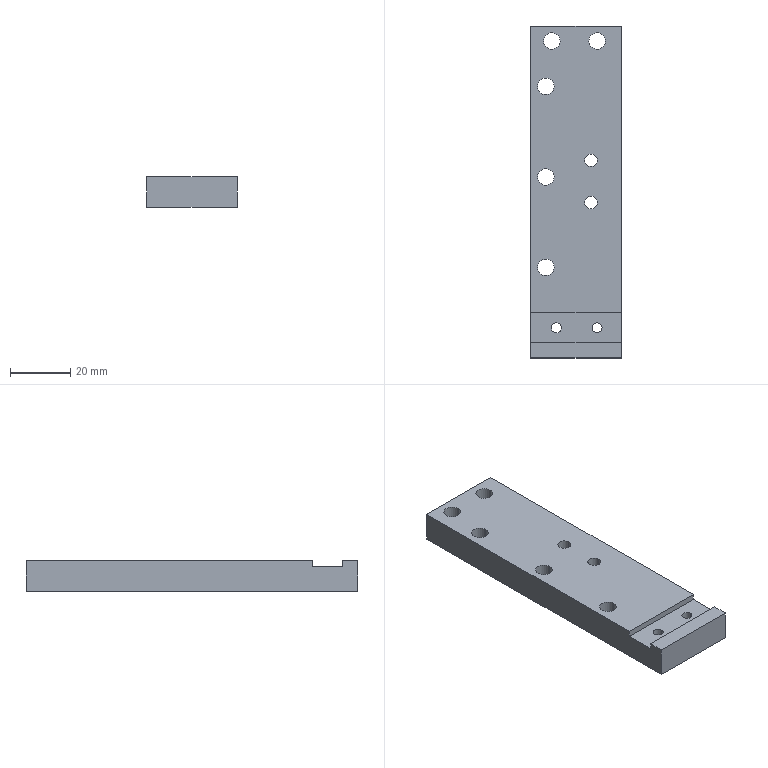Part | NX | features BREP 1 | 1 solid | 28 faces | box 30 x 110 x 10 mm | volume 30798 mm3 | cylinder 18 | plane 10 | commonest cylinder face diameters 5.5 x10 3.3 x4 4.2 x4
STEP:
#1=CARTESIAN_POINT('',(2.903,12.996,0.));
#2=VERTEX_POINT('',#1);
#3=CARTESIAN_POINT('',(7.103,12.996,0.));
#4=VERTEX_POINT('',#3);
#5=CARTESIAN_POINT('',(5.003,12.996,0.));
#6=DIRECTION('',(0.,0.,1.));
#7=DIRECTION('',(1.,0.,0.));
#8=AXIS2_PLACEMENT_3D('',#5,#6,#7);
#9=CIRCLE('',#8,2.1);
#10=EDGE_CURVE('',#2,#4,#9,.T.);
#11=ORIENTED_EDGE('',*,*,#10,.F.);
#12=CARTESIAN_POINT('',(2.903,12.996,10.));
#13=VERTEX_POINT('',#12);
#14=CARTESIAN_POINT('',(2.903,12.996,10.));
#15=DIRECTION('',(0.,0.,1.));
#16=VECTOR('',#15,1000.);
#17=LINE('',#14,#16);
#18=EDGE_CURVE('',#13,#2,#17,.F.);
#19=ORIENTED_EDGE('',*,*,#18,.F.);
#20=CARTESIAN_POINT('',(7.103,12.996,10.));
#21=VERTEX_POINT('',#20);
#22=CARTESIAN_POINT('',(5.003,12.996,10.));
#23=DIRECTION('',(0.,0.,1.));
#24=DIRECTION('',(1.,0.,0.));
#25=AXIS2_PLACEMENT_3D('',#22,#23,#24);
#26=CIRCLE('',#25,2.1);
#27=EDGE_CURVE('',#13,#21,#26,.T.);
#28=ORIENTED_EDGE('',*,*,#27,.T.);
#29=CARTESIAN_POINT('',(7.103,12.996,10.));
#30=DIRECTION('',(0.,0.,1.));
#31=VECTOR('',#30,1000.);
#32=LINE('',#29,#31);
#33=EDGE_CURVE('',#21,#4,#32,.F.);
#34=ORIENTED_EDGE('',*,*,#33,.T.);
#35=EDGE_LOOP('',(#11,#19,#28,#34));
#36=FACE_BOUND('',#35,.T.);
#37=CARTESIAN_POINT('',(5.003,12.996,10.));
#38=DIRECTION('',(0.,0.,1.));
#39=DIRECTION('',(1.,0.,0.));
#40=AXIS2_PLACEMENT_3D('',#37,#38,#39);
#41=CYLINDRICAL_SURFACE('',#40,2.1);
#42=ADVANCED_FACE('',(#36),#41,.F.);
#43=CARTESIAN_POINT('',(2.904,-1.004,0.));
#44=VERTEX_POINT('',#43);
#45=CARTESIAN_POINT('',(7.104,-1.004,0.));
#46=VERTEX_POINT('',#45);
#47=CARTESIAN_POINT('',(5.004,-1.004,0.));
#48=DIRECTION('',(0.,0.,1.));
#49=DIRECTION('',(1.,0.,0.));
#50=AXIS2_PLACEMENT_3D('',#47,#48,#49);
#51=CIRCLE('',#50,2.1);
#52=EDGE_CURVE('',#44,#46,#51,.T.);
#53=ORIENTED_EDGE('',*,*,#52,.F.);
#54=CARTESIAN_POINT('',(2.904,-1.004,10.));
#55=VERTEX_POINT('',#54);
#56=CARTESIAN_POINT('',(2.904,-1.004,10.));
#57=DIRECTION('',(0.,0.,1.));
#58=VECTOR('',#57,1000.);
#59=LINE('',#56,#58);
#60=EDGE_CURVE('',#55,#44,#59,.F.);
#61=ORIENTED_EDGE('',*,*,#60,.F.);
#62=CARTESIAN_POINT('',(7.104,-1.004,10.));
#63=VERTEX_POINT('',#62);
#64=CARTESIAN_POINT('',(5.004,-1.004,10.));
#65=DIRECTION('',(0.,0.,1.));
#66=DIRECTION('',(1.,0.,0.));
#67=AXIS2_PLACEMENT_3D('',#64,#65,#66);
#68=CIRCLE('',#67,2.1);
#69=EDGE_CURVE('',#55,#63,#68,.T.);
#70=ORIENTED_EDGE('',*,*,#69,.T.);
#71=CARTESIAN_POINT('',(7.104,-1.004,10.));
#72=DIRECTION('',(0.,0.,1.));
#73=VECTOR('',#72,1000.);
#74=LINE('',#71,#73);
#75=EDGE_CURVE('',#63,#46,#74,.F.);
#76=ORIENTED_EDGE('',*,*,#75,.T.);
#77=EDGE_LOOP('',(#53,#61,#70,#76));
#78=FACE_BOUND('',#77,.T.);
#79=CARTESIAN_POINT('',(5.004,-1.004,10.));
#80=DIRECTION('',(0.,0.,1.));
#81=DIRECTION('',(1.,0.,0.));
#82=AXIS2_PLACEMENT_3D('',#79,#80,#81);
#83=CYLINDRICAL_SURFACE('',#82,2.1);
#84=ADVANCED_FACE('',(#78),#83,.F.);
#85=CARTESIAN_POINT('',(-12.75,-22.5,0.));
#86=VERTEX_POINT('',#85);
#87=CARTESIAN_POINT('',(-7.25,-22.5,0.));
#88=VERTEX_POINT('',#87);
#89=CARTESIAN_POINT('',(-10.,-22.5,0.));
#90=DIRECTION('',(0.,0.,1.));
#91=DIRECTION('',(1.,0.,0.));
#92=AXIS2_PLACEMENT_3D('',#89,#90,#91);
#93=CIRCLE('',#92,2.75);
#94=EDGE_CURVE('',#86,#88,#93,.T.);
#95=ORIENTED_EDGE('',*,*,#94,.F.);
#96=CARTESIAN_POINT('',(-12.75,-22.5,10.));
#97=VERTEX_POINT('',#96);
#98=CARTESIAN_POINT('',(-12.75,-22.5,0.));
#99=DIRECTION('',(0.,0.,1.));
#100=VECTOR('',#99,1000.);
#101=LINE('',#98,#100);
#102=EDGE_CURVE('',#97,#86,#101,.F.);
#103=ORIENTED_EDGE('',*,*,#102,.F.);
#104=CARTESIAN_POINT('',(-7.25,-22.5,10.));
#105=VERTEX_POINT('',#104);
#106=CARTESIAN_POINT('',(-10.,-22.5,10.));
#107=DIRECTION('',(0.,0.,1.));
#108=DIRECTION('',(1.,0.,0.));
#109=AXIS2_PLACEMENT_3D('',#106,#107,#108);
#110=CIRCLE('',#109,2.75);
#111=EDGE_CURVE('',#97,#105,#110,.T.);
#112=ORIENTED_EDGE('',*,*,#111,.T.);
#113=CARTESIAN_POINT('',(-7.25,-22.5,0.));
#114=DIRECTION('',(0.,0.,1.));
#115=VECTOR('',#114,1000.);
#116=LINE('',#113,#115);
#117=EDGE_CURVE('',#105,#88,#116,.F.);
#118=ORIENTED_EDGE('',*,*,#117,.T.);
#119=EDGE_LOOP('',(#95,#103,#112,#118));
#120=FACE_BOUND('',#119,.T.);
#121=CARTESIAN_POINT('',(-10.,-22.5,0.));
#122=DIRECTION('',(0.,0.,1.));
#123=DIRECTION('',(1.,0.,0.));
#124=AXIS2_PLACEMENT_3D('',#121,#122,#123);
#125=CYLINDRICAL_SURFACE('',#124,2.75);
#126=ADVANCED_FACE('',(#120),#125,.F.);
#127=CARTESIAN_POINT('',(-12.75,7.5,0.));
#128=VERTEX_POINT('',#127);
#129=CARTESIAN_POINT('',(-7.25,7.5,0.));
#130=VERTEX_POINT('',#129);
#131=CARTESIAN_POINT('',(-10.,7.5,0.));
#132=DIRECTION('',(0.,0.,1.));
#133=DIRECTION('',(1.,0.,0.));
#134=AXIS2_PLACEMENT_3D('',#131,#132,#133);
#135=CIRCLE('',#134,2.75);
#136=EDGE_CURVE('',#128,#130,#135,.T.);
#137=ORIENTED_EDGE('',*,*,#136,.F.);
#138=CARTESIAN_POINT('',(-12.75,7.5,10.));
#139=VERTEX_POINT('',#138);
#140=CARTESIAN_POINT('',(-12.75,7.5,0.));
#141=DIRECTION('',(0.,0.,1.));
#142=VECTOR('',#141,1000.);
#143=LINE('',#140,#142);
#144=EDGE_CURVE('',#139,#128,#143,.F.);
#145=ORIENTED_EDGE('',*,*,#144,.F.);
#146=CARTESIAN_POINT('',(-7.25,7.5,10.));
#147=VERTEX_POINT('',#146);
#148=CARTESIAN_POINT('',(-10.,7.5,10.));
#149=DIRECTION('',(0.,0.,1.));
#150=DIRECTION('',(1.,0.,0.));
#151=AXIS2_PLACEMENT_3D('',#148,#149,#150);
#152=CIRCLE('',#151,2.75);
#153=EDGE_CURVE('',#139,#147,#152,.T.);
#154=ORIENTED_EDGE('',*,*,#153,.T.);
#155=CARTESIAN_POINT('',(-7.25,7.5,0.));
#156=DIRECTION('',(0.,0.,1.));
#157=VECTOR('',#156,1000.);
#158=LINE('',#155,#157);
#159=EDGE_CURVE('',#147,#130,#158,.F.);
#160=ORIENTED_EDGE('',*,*,#159,.T.);
#161=EDGE_LOOP('',(#137,#145,#154,#160));
#162=FACE_BOUND('',#161,.T.);
#163=CARTESIAN_POINT('',(-10.,7.5,0.));
#164=DIRECTION('',(0.,0.,1.));
#165=DIRECTION('',(1.,0.,0.));
#166=AXIS2_PLACEMENT_3D('',#163,#164,#165);
#167=CYLINDRICAL_SURFACE('',#166,2.75);
#168=ADVANCED_FACE('',(#162),#167,.F.);
#169=CARTESIAN_POINT('',(-12.75,37.5,0.));
#170=VERTEX_POINT('',#169);
#171=CARTESIAN_POINT('',(-7.25,37.5,0.));
#172=VERTEX_POINT('',#171);
#173=CARTESIAN_POINT('',(-10.,37.5,0.));
#174=DIRECTION('',(0.,0.,1.));
#175=DIRECTION('',(1.,0.,0.));
#176=AXIS2_PLACEMENT_3D('',#173,#174,#175);
#177=CIRCLE('',#176,2.75);
#178=EDGE_CURVE('',#170,#172,#177,.T.);
#179=ORIENTED_EDGE('',*,*,#178,.F.);
#180=CARTESIAN_POINT('',(-12.75,37.5,10.));
#181=VERTEX_POINT('',#180);
#182=CARTESIAN_POINT('',(-12.75,37.5,0.));
#183=DIRECTION('',(0.,0.,1.));
#184=VECTOR('',#183,1000.);
#185=LINE('',#182,#184);
#186=EDGE_CURVE('',#181,#170,#185,.F.);
#187=ORIENTED_EDGE('',*,*,#186,.F.);
#188=CARTESIAN_POINT('',(-7.25,37.5,10.));
#189=VERTEX_POINT('',#188);
#190=CARTESIAN_POINT('',(-10.,37.5,10.));
#191=DIRECTION('',(0.,0.,1.));
#192=DIRECTION('',(1.,0.,0.));
#193=AXIS2_PLACEMENT_3D('',#190,#191,#192);
#194=CIRCLE('',#193,2.75);
#195=EDGE_CURVE('',#181,#189,#194,.T.);
#196=ORIENTED_EDGE('',*,*,#195,.T.);
#197=CARTESIAN_POINT('',(-7.25,37.5,0.));
#198=DIRECTION('',(0.,0.,1.));
#199=VECTOR('',#198,1000.);
#200=LINE('',#197,#199);
#201=EDGE_CURVE('',#189,#172,#200,.F.);
#202=ORIENTED_EDGE('',*,*,#201,.T.);
#203=EDGE_LOOP('',(#179,#187,#196,#202));
#204=FACE_BOUND('',#203,.T.);
#205=CARTESIAN_POINT('',(-10.,37.5,0.));
#206=DIRECTION('',(0.,0.,1.));
#207=DIRECTION('',(1.,0.,0.));
#208=AXIS2_PLACEMENT_3D('',#205,#206,#207);
#209=CYLINDRICAL_SURFACE('',#208,2.75);
#210=ADVANCED_FACE('',(#204),#209,.F.);
#211=CARTESIAN_POINT('',(-8.15,-42.5,0.));
#212=VERTEX_POINT('',#211);
#213=CARTESIAN_POINT('',(-4.85,-42.5,0.));
#214=VERTEX_POINT('',#213);
#215=CARTESIAN_POINT('',(-6.5,-42.5,0.));
#216=DIRECTION('',(0.,0.,1.));
#217=DIRECTION('',(1.,0.,0.));
#218=AXIS2_PLACEMENT_3D('',#215,#216,#217);
#219=CIRCLE('',#218,1.65);
#220=EDGE_CURVE('',#212,#214,#219,.T.);
#221=ORIENTED_EDGE('',*,*,#220,.F.);
#222=CARTESIAN_POINT('',(-8.15,-42.5,8.));
#223=VERTEX_POINT('',#222);
#224=CARTESIAN_POINT('',(-8.15,-42.5,8.));
#225=DIRECTION('',(0.,0.,1.));
#226=VECTOR('',#225,1000.);
#227=LINE('',#224,#226);
#228=EDGE_CURVE('',#223,#212,#227,.F.);
#229=ORIENTED_EDGE('',*,*,#228,.F.);
#230=CARTESIAN_POINT('',(-4.85,-42.5,8.));
#231=VERTEX_POINT('',#230);
#232=CARTESIAN_POINT('',(-6.5,-42.5,8.));
#233=DIRECTION('',(0.,0.,1.));
#234=DIRECTION('',(1.,0.,0.));
#235=AXIS2_PLACEMENT_3D('',#232,#233,#234);
#236=CIRCLE('',#235,1.65);
#237=EDGE_CURVE('',#223,#231,#236,.T.);
#238=ORIENTED_EDGE('',*,*,#237,.T.);
#239=CARTESIAN_POINT('',(-4.85,-42.5,8.));
#240=DIRECTION('',(0.,0.,1.));
#241=VECTOR('',#240,1000.);
#242=LINE('',#239,#241);
#243=EDGE_CURVE('',#231,#214,#242,.F.);
#244=ORIENTED_EDGE('',*,*,#243,.T.);
#245=EDGE_LOOP('',(#221,#229,#238,#244));
#246=FACE_BOUND('',#245,.T.);
#247=CARTESIAN_POINT('',(-6.5,-42.5,8.));
#248=DIRECTION('',(0.,0.,1.));
#249=DIRECTION('',(1.,0.,0.));
#250=AXIS2_PLACEMENT_3D('',#247,#248,#249);
#251=CYLINDRICAL_SURFACE('',#250,1.65);
#252=ADVANCED_FACE('',(#246),#251,.F.);
#253=CARTESIAN_POINT('',(5.35,-42.5,0.));
#254=VERTEX_POINT('',#253);
#255=CARTESIAN_POINT('',(8.65,-42.5,0.));
#256=VERTEX_POINT('',#255);
#257=CARTESIAN_POINT('',(7.,-42.5,0.));
#258=DIRECTION('',(0.,0.,1.));
#259=DIRECTION('',(1.,0.,0.));
#260=AXIS2_PLACEMENT_3D('',#257,#258,#259);
#261=CIRCLE('',#260,1.65);
#262=EDGE_CURVE('',#254,#256,#261,.T.);
#263=ORIENTED_EDGE('',*,*,#262,.F.);
#264=CARTESIAN_POINT('',(5.35,-42.5,8.));
#265=VERTEX_POINT('',#264);
#266=CARTESIAN_POINT('',(5.35,-42.5,8.));
#267=DIRECTION('',(0.,0.,1.));
#268=VECTOR('',#267,1000.);
#269=LINE('',#266,#268);
#270=EDGE_CURVE('',#265,#254,#269,.F.);
#271=ORIENTED_EDGE('',*,*,#270,.F.);
#272=CARTESIAN_POINT('',(8.65,-42.5,8.));
#273=VERTEX_POINT('',#272);
#274=CARTESIAN_POINT('',(7.,-42.5,8.));
#275=DIRECTION('',(0.,0.,1.));
#276=DIRECTION('',(1.,0.,0.));
#277=AXIS2_PLACEMENT_3D('',#274,#275,#276);
#278=CIRCLE('',#277,1.65);
#279=EDGE_CURVE('',#265,#273,#278,.T.);
#280=ORIENTED_EDGE('',*,*,#279,.T.);
#281=CARTESIAN_POINT('',(8.65,-42.5,8.));
#282=DIRECTION('',(0.,0.,1.));
#283=VECTOR('',#282,1000.);
#284=LINE('',#281,#283);
#285=EDGE_CURVE('',#273,#256,#284,.F.);
#286=ORIENTED_EDGE('',*,*,#285,.T.);
#287=EDGE_LOOP('',(#263,#271,#280,#286));
#288=FACE_BOUND('',#287,.T.);
#289=CARTESIAN_POINT('',(7.,-42.5,8.));
#290=DIRECTION('',(0.,0.,1.));
#291=DIRECTION('',(1.,0.,0.));
#292=AXIS2_PLACEMENT_3D('',#289,#290,#291);
#293=CYLINDRICAL_SURFACE('',#292,1.65);
#294=ADVANCED_FACE('',(#288),#293,.F.);
#295=CARTESIAN_POINT('',(4.25,52.5,0.));
#296=VERTEX_POINT('',#295);
#297=CARTESIAN_POINT('',(9.75,52.5,0.));
#298=VERTEX_POINT('',#297);
#299=CARTESIAN_POINT('',(7.,52.5,0.));
#300=DIRECTION('',(0.,0.,1.));
#301=DIRECTION('',(1.,0.,0.));
#302=AXIS2_PLACEMENT_3D('',#299,#300,#301);
#303=CIRCLE('',#302,2.75);
#304=EDGE_CURVE('',#296,#298,#303,.T.);
#305=ORIENTED_EDGE('',*,*,#304,.F.);
#306=CARTESIAN_POINT('',(4.25,52.5,10.));
#307=VERTEX_POINT('',#306);
#308=CARTESIAN_POINT('',(4.25,52.5,0.));
#309=DIRECTION('',(0.,0.,1.));
#310=VECTOR('',#309,1000.);
#311=LINE('',#308,#310);
#312=EDGE_CURVE('',#307,#296,#311,.F.);
#313=ORIENTED_EDGE('',*,*,#312,.F.);
#314=CARTESIAN_POINT('',(9.75,52.5,10.));
#315=VERTEX_POINT('',#314);
#316=CARTESIAN_POINT('',(7.,52.5,10.));
#317=DIRECTION('',(0.,0.,1.));
#318=DIRECTION('',(1.,0.,0.));
#319=AXIS2_PLACEMENT_3D('',#316,#317,#318);
#320=CIRCLE('',#319,2.75);
#321=EDGE_CURVE('',#307,#315,#320,.T.);
#322=ORIENTED_EDGE('',*,*,#321,.T.);
#323=CARTESIAN_POINT('',(9.75,52.5,0.));
#324=DIRECTION('',(0.,0.,1.));
#325=VECTOR('',#324,1000.);
#326=LINE('',#323,#325);
#327=EDGE_CURVE('',#315,#298,#326,.F.);
#328=ORIENTED_EDGE('',*,*,#327,.T.);
#329=EDGE_LOOP('',(#305,#313,#322,#328));
#330=FACE_BOUND('',#329,.T.);
#331=CARTESIAN_POINT('',(7.,52.5,0.));
#332=DIRECTION('',(0.,0.,1.));
#333=DIRECTION('',(1.,0.,0.));
#334=AXIS2_PLACEMENT_3D('',#331,#332,#333);
#335=CYLINDRICAL_SURFACE('',#334,2.75);
#336=ADVANCED_FACE('',(#330),#335,.F.);
#337=CARTESIAN_POINT('',(-10.75,52.5,0.));
#338=VERTEX_POINT('',#337);
#339=CARTESIAN_POINT('',(-5.25,52.5,0.));
#340=VERTEX_POINT('',#339);
#341=CARTESIAN_POINT('',(-8.,52.5,0.));
#342=DIRECTION('',(0.,0.,1.));
#343=DIRECTION('',(1.,0.,0.));
#344=AXIS2_PLACEMENT_3D('',#341,#342,#343);
#345=CIRCLE('',#344,2.75);
#346=EDGE_CURVE('',#338,#340,#345,.T.);
#347=ORIENTED_EDGE('',*,*,#346,.F.);
#348=CARTESIAN_POINT('',(-10.75,52.5,10.));
#349=VERTEX_POINT('',#348);
#350=CARTESIAN_POINT('',(-10.75,52.5,0.));
#351=DIRECTION('',(0.,0.,1.));
#352=VECTOR('',#351,1000.);
#353=LINE('',#350,#352);
#354=EDGE_CURVE('',#349,#338,#353,.F.);
#355=ORIENTED_EDGE('',*,*,#354,.F.);
#356=CARTESIAN_POINT('',(-5.25,52.5,10.));
#357=VERTEX_POINT('',#356);
#358=CARTESIAN_POINT('',(-8.,52.5,10.));
#359=DIRECTION('',(0.,0.,1.));
#360=DIRECTION('',(1.,0.,0.));
#361=AXIS2_PLACEMENT_3D('',#358,#359,#360);
#362=CIRCLE('',#361,2.75);
#363=EDGE_CURVE('',#349,#357,#362,.T.);
#364=ORIENTED_EDGE('',*,*,#363,.T.);
#365=CARTESIAN_POINT('',(-5.25,52.5,0.));
#366=DIRECTION('',(0.,0.,1.));
#367=VECTOR('',#366,1000.);
#368=LINE('',#365,#367);
#369=EDGE_CURVE('',#357,#340,#368,.F.);
#370=ORIENTED_EDGE('',*,*,#369,.T.);
#371=EDGE_LOOP('',(#347,#355,#364,#370));
#372=FACE_BOUND('',#371,.T.);
#373=CARTESIAN_POINT('',(-8.,52.5,0.));
#374=DIRECTION('',(0.,0.,1.));
#375=DIRECTION('',(1.,0.,0.));
#376=AXIS2_PLACEMENT_3D('',#373,#374,#375);
#377=CYLINDRICAL_SURFACE('',#376,2.75);
#378=ADVANCED_FACE('',(#372),#377,.F.);
#379=CARTESIAN_POINT('',(15.,-37.5,10.));
#380=VERTEX_POINT('',#379);
#381=CARTESIAN_POINT('',(-15.,-37.5,10.));
#382=VERTEX_POINT('',#381);
#383=CARTESIAN_POINT('',(-15.,-37.5,10.));
#384=DIRECTION('',(-1.,0.,0.));
#385=VECTOR('',#384,1000.);
#386=LINE('',#383,#385);
#387=EDGE_CURVE('',#380,#382,#386,.T.);
#388=ORIENTED_EDGE('',*,*,#387,.F.);
#389=CARTESIAN_POINT('',(15.,57.5,10.));
#390=VERTEX_POINT('',#389);
#391=CARTESIAN_POINT('',(15.,57.5,10.));
#392=DIRECTION('',(0.,1.,0.));
#393=VECTOR('',#392,1000.);
#394=LINE('',#391,#393);
#395=EDGE_CURVE('',#380,#390,#394,.T.);
#396=ORIENTED_EDGE('',*,*,#395,.T.);
#397=CARTESIAN_POINT('',(-15.,57.5,10.));
#398=VERTEX_POINT('',#397);
#399=CARTESIAN_POINT('',(-15.,57.5,10.));
#400=DIRECTION('',(-1.,0.,0.));
#401=VECTOR('',#400,1000.);
#402=LINE('',#399,#401);
#403=EDGE_CURVE('',#390,#398,#402,.T.);
#404=ORIENTED_EDGE('',*,*,#403,.T.);
#405=CARTESIAN_POINT('',(-15.,57.5,10.));
#406=DIRECTION('',(0.,-1.,0.));
#407=VECTOR('',#406,1000.);
#408=LINE('',#405,#407);
#409=EDGE_CURVE('',#398,#382,#408,.T.);
#410=ORIENTED_EDGE('',*,*,#409,.T.);
#411=EDGE_LOOP('',(#388,#396,#404,#410));
#412=FACE_BOUND('',#411,.T.);
#413=CARTESIAN_POINT('',(5.003,12.996,10.));
#414=DIRECTION('',(0.,0.,1.));
#415=DIRECTION('',(1.,0.,0.));
#416=AXIS2_PLACEMENT_3D('',#413,#414,#415);
#417=CIRCLE('',#416,2.1);
#418=EDGE_CURVE('',#21,#13,#417,.T.);
#419=ORIENTED_EDGE('',*,*,#418,.F.);
#420=ORIENTED_EDGE('',*,*,#27,.F.);
#421=EDGE_LOOP('',(#419,#420));
#422=FACE_BOUND('',#421,.T.);
#423=CARTESIAN_POINT('',(5.004,-1.004,10.));
#424=DIRECTION('',(0.,0.,1.));
#425=DIRECTION('',(1.,0.,0.));
#426=AXIS2_PLACEMENT_3D('',#423,#424,#425);
#427=CIRCLE('',#426,2.1);
#428=EDGE_CURVE('',#63,#55,#427,.T.);
#429=ORIENTED_EDGE('',*,*,#428,.F.);
#430=ORIENTED_EDGE('',*,*,#69,.F.);
#431=EDGE_LOOP('',(#429,#430));
#432=FACE_BOUND('',#431,.T.);
#433=CARTESIAN_POINT('',(-10.,-22.5,10.));
#434=DIRECTION('',(0.,0.,1.));
#435=DIRECTION('',(1.,0.,0.));
#436=AXIS2_PLACEMENT_3D('',#433,#434,#435);
#437=CIRCLE('',#436,2.75);
#438=EDGE_CURVE('',#105,#97,#437,.T.);
#439=ORIENTED_EDGE('',*,*,#438,.F.);
#440=ORIENTED_EDGE('',*,*,#111,.F.);
#441=EDGE_LOOP('',(#439,#440));
#442=FACE_BOUND('',#441,.T.);
#443=CARTESIAN_POINT('',(-10.,7.5,10.));
#444=DIRECTION('',(0.,0.,1.));
#445=DIRECTION('',(1.,0.,0.));
#446=AXIS2_PLACEMENT_3D('',#443,#444,#445);
#447=CIRCLE('',#446,2.75);
#448=EDGE_CURVE('',#147,#139,#447,.T.);
#449=ORIENTED_EDGE('',*,*,#448,.F.);
#450=ORIENTED_EDGE('',*,*,#153,.F.);
#451=EDGE_LOOP('',(#449,#450));
#452=FACE_BOUND('',#451,.T.);
#453=CARTESIAN_POINT('',(-10.,37.5,10.));
#454=DIRECTION('',(0.,0.,1.));
#455=DIRECTION('',(1.,0.,0.));
#456=AXIS2_PLACEMENT_3D('',#453,#454,#455);
#457=CIRCLE('',#456,2.75);
#458=EDGE_CURVE('',#189,#181,#457,.T.);
#459=ORIENTED_EDGE('',*,*,#458,.F.);
#460=ORIENTED_EDGE('',*,*,#195,.F.);
#461=EDGE_LOOP('',(#459,#460));
#462=FACE_BOUND('',#461,.T.);
#463=CARTESIAN_POINT('',(7.,52.5,10.));
#464=DIRECTION('',(0.,0.,1.));
#465=DIRECTION('',(1.,0.,0.));
#466=AXIS2_PLACEMENT_3D('',#463,#464,#465);
#467=CIRCLE('',#466,2.75);
#468=EDGE_CURVE('',#315,#307,#467,.T.);
#469=ORIENTED_EDGE('',*,*,#468,.F.);
#470=ORIENTED_EDGE('',*,*,#321,.F.);
#471=EDGE_LOOP('',(#469,#470));
#472=FACE_BOUND('',#471,.T.);
#473=CARTESIAN_POINT('',(-8.,52.5,10.));
#474=DIRECTION('',(0.,0.,1.));
#475=DIRECTION('',(1.,0.,0.));
#476=AXIS2_PLACEMENT_3D('',#473,#474,#475);
#477=CIRCLE('',#476,2.75);
#478=EDGE_CURVE('',#357,#349,#477,.T.);
#479=ORIENTED_EDGE('',*,*,#478,.F.);
#480=ORIENTED_EDGE('',*,*,#363,.F.);
#481=EDGE_LOOP('',(#479,#480));
#482=FACE_BOUND('',#481,.T.);
#483=CARTESIAN_POINT('',(-15.,-52.5,10.));
#484=DIRECTION('',(0.,0.,1.));
#485=DIRECTION('',(1.,0.,0.));
#486=AXIS2_PLACEMENT_3D('',#483,#484,#485);
#487=PLANE('',#486);
#488=ADVANCED_FACE('',(#412,#422,#432,#442,#452,#462,#472,#482),#487,.T.);
#489=CARTESIAN_POINT('',(-15.,-37.5,8.));
#490=VERTEX_POINT('',#489);
#491=CARTESIAN_POINT('',(-15.,-47.5,8.));
#492=VERTEX_POINT('',#491);
#493=CARTESIAN_POINT('',(-15.,-37.5,8.));
#494=DIRECTION('',(0.,-1.,0.));
#495=VECTOR('',#494,1000.);
#496=LINE('',#493,#495);
#497=EDGE_CURVE('',#490,#492,#496,.T.);
#498=ORIENTED_EDGE('',*,*,#497,.F.);
#499=CARTESIAN_POINT('',(-15.,-37.5,8.));
#500=DIRECTION('',(0.,0.,1.));
#501=VECTOR('',#500,1000.);
#502=LINE('',#499,#501);
#503=EDGE_CURVE('',#490,#382,#502,.T.);
#504=ORIENTED_EDGE('',*,*,#503,.T.);
#505=ORIENTED_EDGE('',*,*,#409,.F.);
#506=CARTESIAN_POINT('',(-15.,57.5,0.));
#507=VERTEX_POINT('',#506);
#508=CARTESIAN_POINT('',(-15.,57.5,10.));
#509=DIRECTION('',(0.,0.,-1.));
#510=VECTOR('',#509,1000.);
#511=LINE('',#508,#510);
#512=EDGE_CURVE('',#398,#507,#511,.T.);
#513=ORIENTED_EDGE('',*,*,#512,.T.);
#514=CARTESIAN_POINT('',(-15.,-52.5,0.));
#515=VERTEX_POINT('',#514);
#516=CARTESIAN_POINT('',(-15.,57.5,0.));
#517=DIRECTION('',(0.,-1.,0.));
#518=VECTOR('',#517,1000.);
#519=LINE('',#516,#518);
#520=EDGE_CURVE('',#507,#515,#519,.T.);
#521=ORIENTED_EDGE('',*,*,#520,.T.);
#522=CARTESIAN_POINT('',(-15.,-52.5,10.));
#523=VERTEX_POINT('',#522);
#524=CARTESIAN_POINT('',(-15.,-52.5,10.));
#525=DIRECTION('',(0.,0.,-1.));
#526=VECTOR('',#525,1000.);
#527=LINE('',#524,#526);
#528=EDGE_CURVE('',#523,#515,#527,.T.);
#529=ORIENTED_EDGE('',*,*,#528,.F.);
#530=CARTESIAN_POINT('',(-15.,-47.5,10.));
#531=VERTEX_POINT('',#530);
#532=CARTESIAN_POINT('',(-15.,57.5,10.));
#533=DIRECTION('',(0.,-1.,0.));
#534=VECTOR('',#533,1000.);
#535=LINE('',#532,#534);
#536=EDGE_CURVE('',#531,#523,#535,.T.);
#537=ORIENTED_EDGE('',*,*,#536,.F.);
#538=CARTESIAN_POINT('',(-15.,-47.5,8.));
#539=DIRECTION('',(0.,0.,1.));
#540=VECTOR('',#539,1000.);
#541=LINE('',#538,#540);
#542=EDGE_CURVE('',#492,#531,#541,.T.);
#543=ORIENTED_EDGE('',*,*,#542,.F.);
#544=EDGE_LOOP('',(#498,#504,#505,#513,#521,#529,#537,#543));
#545=FACE_BOUND('',#544,.T.);
#546=CARTESIAN_POINT('',(-15.,57.5,10.));
#547=DIRECTION('',(1.,0.,0.));
#548=DIRECTION('',(0.,1.,0.));
#549=AXIS2_PLACEMENT_3D('',#546,#547,#548);
#550=PLANE('',#549);
#551=ADVANCED_FACE('',(#545),#550,.F.);
#552=CARTESIAN_POINT('',(15.,-52.5,0.));
#553=VERTEX_POINT('',#552);
#554=CARTESIAN_POINT('',(-15.,-52.5,0.));
#555=DIRECTION('',(1.,0.,0.));
#556=VECTOR('',#555,1000.);
#557=LINE('',#554,#556);
#558=EDGE_CURVE('',#515,#553,#557,.T.);
#559=ORIENTED_EDGE('',*,*,#558,.T.);
#560=CARTESIAN_POINT('',(15.,-52.5,10.));
#561=VERTEX_POINT('',#560);
#562=CARTESIAN_POINT('',(15.,-52.5,10.));
#563=DIRECTION('',(0.,0.,-1.));
#564=VECTOR('',#563,1000.);
#565=LINE('',#562,#564);
#566=EDGE_CURVE('',#561,#553,#565,.T.);
#567=ORIENTED_EDGE('',*,*,#566,.F.);
#568=CARTESIAN_POINT('',(-15.,-52.5,10.));
#569=DIRECTION('',(1.,0.,0.));
#570=VECTOR('',#569,1000.);
#571=LINE('',#568,#570);
#572=EDGE_CURVE('',#523,#561,#571,.T.);
#573=ORIENTED_EDGE('',*,*,#572,.F.);
#574=ORIENTED_EDGE('',*,*,#528,.T.);
#575=EDGE_LOOP('',(#559,#567,#573,#574));
#576=FACE_BOUND('',#575,.T.);
#577=CARTESIAN_POINT('',(-15.,-52.5,10.));
#578=DIRECTION('',(0.,1.,0.));
#579=DIRECTION('',(1.,0.,0.));
#580=AXIS2_PLACEMENT_3D('',#577,#578,#579);
#581=PLANE('',#580);
#582=ADVANCED_FACE('',(#576),#581,.F.);
#583=ORIENTED_EDGE('',*,*,#395,.F.);
#584=CARTESIAN_POINT('',(15.,-37.5,8.));
#585=VERTEX_POINT('',#584);
#586=CARTESIAN_POINT('',(15.,-37.5,8.));
#587=DIRECTION('',(0.,0.,1.));
#588=VECTOR('',#587,1000.);
#589=LINE('',#586,#588);
#590=EDGE_CURVE('',#585,#380,#589,.T.);
#591=ORIENTED_EDGE('',*,*,#590,.F.);
#592=CARTESIAN_POINT('',(15.,-47.5,8.));
#593=VERTEX_POINT('',#592);
#594=CARTESIAN_POINT('',(15.,-37.5,8.));
#595=DIRECTION('',(0.,1.,0.));
#596=VECTOR('',#595,1000.);
#597=LINE('',#594,#596);
#598=EDGE_CURVE('',#593,#585,#597,.T.);
#599=ORIENTED_EDGE('',*,*,#598,.F.);
#600=CARTESIAN_POINT('',(15.,-47.5,10.));
#601=VERTEX_POINT('',#600);
#602=CARTESIAN_POINT('',(15.,-47.5,8.));
#603=DIRECTION('',(0.,0.,1.));
#604=VECTOR('',#603,1000.);
#605=LINE('',#602,#604);
#606=EDGE_CURVE('',#593,#601,#605,.T.);
#607=ORIENTED_EDGE('',*,*,#606,.T.);
#608=CARTESIAN_POINT('',(15.,57.5,10.));
#609=DIRECTION('',(0.,1.,0.));
#610=VECTOR('',#609,1000.);
#611=LINE('',#608,#610);
#612=EDGE_CURVE('',#561,#601,#611,.T.);
#613=ORIENTED_EDGE('',*,*,#612,.F.);
#614=ORIENTED_EDGE('',*,*,#566,.T.);
#615=CARTESIAN_POINT('',(15.,57.5,0.));
#616=VERTEX_POINT('',#615);
#617=CARTESIAN_POINT('',(15.,57.5,0.));
#618=DIRECTION('',(0.,1.,0.));
#619=VECTOR('',#618,1000.);
#620=LINE('',#617,#619);
#621=EDGE_CURVE('',#553,#616,#620,.T.);
#622=ORIENTED_EDGE('',*,*,#621,.T.);
#623=CARTESIAN_POINT('',(15.,57.5,10.));
#624=DIRECTION('',(0.,0.,-1.));
#625=VECTOR('',#624,1000.);
#626=LINE('',#623,#625);
#627=EDGE_CURVE('',#390,#616,#626,.T.);
#628=ORIENTED_EDGE('',*,*,#627,.F.);
#629=EDGE_LOOP('',(#583,#591,#599,#607,#613,#614,#622,#628));
#630=FACE_BOUND('',#629,.T.);
#631=CARTESIAN_POINT('',(15.,57.5,10.));
#632=DIRECTION('',(-1.,0.,0.));
#633=DIRECTION('',(0.,1.,0.));
#634=AXIS2_PLACEMENT_3D('',#631,#632,#633);
#635=PLANE('',#634);
#636=ADVANCED_FACE('',(#630),#635,.F.);
#637=CARTESIAN_POINT('',(-15.,57.5,0.));
#638=DIRECTION('',(-1.,0.,0.));
#639=VECTOR('',#638,1000.);
#640=LINE('',#637,#639);
#641=EDGE_CURVE('',#616,#507,#640,.T.);
#642=ORIENTED_EDGE('',*,*,#641,.T.);
#643=ORIENTED_EDGE('',*,*,#512,.F.);
#644=ORIENTED_EDGE('',*,*,#403,.F.);
#645=ORIENTED_EDGE('',*,*,#627,.T.);
#646=EDGE_LOOP('',(#642,#643,#644,#645));
#647=FACE_BOUND('',#646,.T.);
#648=CARTESIAN_POINT('',(-15.,57.5,10.));
#649=DIRECTION('',(0.,-1.,0.));
#650=DIRECTION('',(0.,0.,-1.));
#651=AXIS2_PLACEMENT_3D('',#648,#649,#650);
#652=PLANE('',#651);
#653=ADVANCED_FACE('',(#647),#652,.F.);
#654=CARTESIAN_POINT('',(-15.,-47.5,10.));
#655=DIRECTION('',(1.,0.,0.));
#656=VECTOR('',#655,1000.);
#657=LINE('',#654,#656);
#658=EDGE_CURVE('',#531,#601,#657,.T.);
#659=ORIENTED_EDGE('',*,*,#658,.F.);
#660=ORIENTED_EDGE('',*,*,#536,.T.);
#661=ORIENTED_EDGE('',*,*,#572,.T.);
#662=ORIENTED_EDGE('',*,*,#612,.T.);
#663=EDGE_LOOP('',(#659,#660,#661,#662));
#664=FACE_BOUND('',#663,.T.);
#665=CARTESIAN_POINT('',(-15.,-52.5,10.));
#666=DIRECTION('',(0.,0.,1.));
#667=DIRECTION('',(1.,0.,0.));
#668=AXIS2_PLACEMENT_3D('',#665,#666,#667);
#669=PLANE('',#668);
#670=ADVANCED_FACE('',(#664),#669,.T.);
#671=ORIENTED_EDGE('',*,*,#520,.F.);
#672=ORIENTED_EDGE('',*,*,#641,.F.);
#673=ORIENTED_EDGE('',*,*,#621,.F.);
#674=ORIENTED_EDGE('',*,*,#558,.F.);
#675=EDGE_LOOP('',(#671,#672,#673,#674));
#676=FACE_BOUND('',#675,.T.);
#677=CARTESIAN_POINT('',(5.003,12.996,0.));
#678=DIRECTION('',(0.,0.,1.));
#679=DIRECTION('',(1.,0.,0.));
#680=AXIS2_PLACEMENT_3D('',#677,#678,#679);
#681=CIRCLE('',#680,2.1);
#682=EDGE_CURVE('',#4,#2,#681,.T.);
#683=ORIENTED_EDGE('',*,*,#682,.T.);
#684=ORIENTED_EDGE('',*,*,#10,.T.);
#685=EDGE_LOOP('',(#683,#684));
#686=FACE_BOUND('',#685,.T.);
#687=CARTESIAN_POINT('',(5.004,-1.004,0.));
#688=DIRECTION('',(0.,0.,1.));
#689=DIRECTION('',(1.,0.,0.));
#690=AXIS2_PLACEMENT_3D('',#687,#688,#689);
#691=CIRCLE('',#690,2.1);
#692=EDGE_CURVE('',#46,#44,#691,.T.);
#693=ORIENTED_EDGE('',*,*,#692,.T.);
#694=ORIENTED_EDGE('',*,*,#52,.T.);
#695=EDGE_LOOP('',(#693,#694));
#696=FACE_BOUND('',#695,.T.);
#697=CARTESIAN_POINT('',(-10.,-22.5,0.));
#698=DIRECTION('',(0.,0.,1.));
#699=DIRECTION('',(1.,0.,0.));
#700=AXIS2_PLACEMENT_3D('',#697,#698,#699);
#701=CIRCLE('',#700,2.75);
#702=EDGE_CURVE('',#88,#86,#701,.T.);
#703=ORIENTED_EDGE('',*,*,#702,.T.);
#704=ORIENTED_EDGE('',*,*,#94,.T.);
#705=EDGE_LOOP('',(#703,#704));
#706=FACE_BOUND('',#705,.T.);
#707=CARTESIAN_POINT('',(-10.,7.5,0.));
#708=DIRECTION('',(0.,0.,1.));
#709=DIRECTION('',(1.,0.,0.));
#710=AXIS2_PLACEMENT_3D('',#707,#708,#709);
#711=CIRCLE('',#710,2.75);
#712=EDGE_CURVE('',#130,#128,#711,.T.);
#713=ORIENTED_EDGE('',*,*,#712,.T.);
#714=ORIENTED_EDGE('',*,*,#136,.T.);
#715=EDGE_LOOP('',(#713,#714));
#716=FACE_BOUND('',#715,.T.);
#717=CARTESIAN_POINT('',(-10.,37.5,0.));
#718=DIRECTION('',(0.,0.,1.));
#719=DIRECTION('',(1.,0.,0.));
#720=AXIS2_PLACEMENT_3D('',#717,#718,#719);
#721=CIRCLE('',#720,2.75);
#722=EDGE_CURVE('',#172,#170,#721,.T.);
#723=ORIENTED_EDGE('',*,*,#722,.T.);
#724=ORIENTED_EDGE('',*,*,#178,.T.);
#725=EDGE_LOOP('',(#723,#724));
#726=FACE_BOUND('',#725,.T.);
#727=CARTESIAN_POINT('',(-6.5,-42.5,0.));
#728=DIRECTION('',(0.,0.,1.));
#729=DIRECTION('',(1.,0.,0.));
#730=AXIS2_PLACEMENT_3D('',#727,#728,#729);
#731=CIRCLE('',#730,1.65);
#732=EDGE_CURVE('',#214,#212,#731,.T.);
#733=ORIENTED_EDGE('',*,*,#732,.T.);
#734=ORIENTED_EDGE('',*,*,#220,.T.);
#735=EDGE_LOOP('',(#733,#734));
#736=FACE_BOUND('',#735,.T.);
#737=CARTESIAN_POINT('',(7.,-42.5,0.));
#738=DIRECTION('',(0.,0.,1.));
#739=DIRECTION('',(1.,0.,0.));
#740=AXIS2_PLACEMENT_3D('',#737,#738,#739);
#741=CIRCLE('',#740,1.65);
#742=EDGE_CURVE('',#256,#254,#741,.T.);
#743=ORIENTED_EDGE('',*,*,#742,.T.);
#744=ORIENTED_EDGE('',*,*,#262,.T.);
#745=EDGE_LOOP('',(#743,#744));
#746=FACE_BOUND('',#745,.T.);
#747=CARTESIAN_POINT('',(7.,52.5,0.));
#748=DIRECTION('',(0.,0.,1.));
#749=DIRECTION('',(1.,0.,0.));
#750=AXIS2_PLACEMENT_3D('',#747,#748,#749);
#751=CIRCLE('',#750,2.75);
#752=EDGE_CURVE('',#298,#296,#751,.T.);
#753=ORIENTED_EDGE('',*,*,#752,.T.);
#754=ORIENTED_EDGE('',*,*,#304,.T.);
#755=EDGE_LOOP('',(#753,#754));
#756=FACE_BOUND('',#755,.T.);
#757=CARTESIAN_POINT('',(-8.,52.5,0.));
#758=DIRECTION('',(0.,0.,1.));
#759=DIRECTION('',(1.,0.,0.));
#760=AXIS2_PLACEMENT_3D('',#757,#758,#759);
#761=CIRCLE('',#760,2.75);
#762=EDGE_CURVE('',#340,#338,#761,.T.);
#763=ORIENTED_EDGE('',*,*,#762,.T.);
#764=ORIENTED_EDGE('',*,*,#346,.T.);
#765=EDGE_LOOP('',(#763,#764));
#766=FACE_BOUND('',#765,.T.);
#767=CARTESIAN_POINT('',(-15.,-52.5,0.));
#768=DIRECTION('',(0.,0.,1.));
#769=DIRECTION('',(1.,0.,0.));
#770=AXIS2_PLACEMENT_3D('',#767,#768,#769);
#771=PLANE('',#770);
#772=ADVANCED_FACE('',(#676,#686,#696,#706,#716,#726,#736,#746,#756,#766),#771,.F.);
#773=ORIENTED_EDGE('',*,*,#387,.T.);
#774=ORIENTED_EDGE('',*,*,#503,.F.);
#775=CARTESIAN_POINT('',(-15.,-37.5,8.));
#776=DIRECTION('',(-1.,0.,0.));
#777=VECTOR('',#776,1000.);
#778=LINE('',#775,#777);
#779=EDGE_CURVE('',#585,#490,#778,.T.);
#780=ORIENTED_EDGE('',*,*,#779,.F.);
#781=ORIENTED_EDGE('',*,*,#590,.T.);
#782=EDGE_LOOP('',(#773,#774,#780,#781));
#783=FACE_BOUND('',#782,.T.);
#784=CARTESIAN_POINT('',(-15.,-37.5,8.));
#785=DIRECTION('',(0.,1.,0.));
#786=DIRECTION('',(1.,0.,0.));
#787=AXIS2_PLACEMENT_3D('',#784,#785,#786);
#788=PLANE('',#787);
#789=ADVANCED_FACE('',(#783),#788,.F.);
#790=ORIENTED_EDGE('',*,*,#658,.T.);
#791=ORIENTED_EDGE('',*,*,#606,.F.);
#792=CARTESIAN_POINT('',(-15.,-47.5,8.));
#793=DIRECTION('',(1.,0.,0.));
#794=VECTOR('',#793,1000.);
#795=LINE('',#792,#794);
#796=EDGE_CURVE('',#492,#593,#795,.T.);
#797=ORIENTED_EDGE('',*,*,#796,.F.);
#798=ORIENTED_EDGE('',*,*,#542,.T.);
#799=EDGE_LOOP('',(#790,#791,#797,#798));
#800=FACE_BOUND('',#799,.T.);
#801=CARTESIAN_POINT('',(-15.,-47.5,8.));
#802=DIRECTION('',(0.,-1.,0.));
#803=DIRECTION('',(0.,0.,-1.));
#804=AXIS2_PLACEMENT_3D('',#801,#802,#803);
#805=PLANE('',#804);
#806=ADVANCED_FACE('',(#800),#805,.F.);
#807=ORIENTED_EDGE('',*,*,#497,.T.);
#808=ORIENTED_EDGE('',*,*,#796,.T.);
#809=ORIENTED_EDGE('',*,*,#598,.T.);
#810=ORIENTED_EDGE('',*,*,#779,.T.);
#811=EDGE_LOOP('',(#807,#808,#809,#810));
#812=FACE_BOUND('',#811,.T.);
#813=CARTESIAN_POINT('',(-6.5,-42.5,8.));
#814=DIRECTION('',(0.,0.,1.));
#815=DIRECTION('',(1.,0.,0.));
#816=AXIS2_PLACEMENT_3D('',#813,#814,#815);
#817=CIRCLE('',#816,1.65);
#818=EDGE_CURVE('',#231,#223,#817,.T.);
#819=ORIENTED_EDGE('',*,*,#818,.F.);
#820=ORIENTED_EDGE('',*,*,#237,.F.);
#821=EDGE_LOOP('',(#819,#820));
#822=FACE_BOUND('',#821,.T.);
#823=CARTESIAN_POINT('',(7.,-42.5,8.));
#824=DIRECTION('',(0.,0.,1.));
#825=DIRECTION('',(1.,0.,0.));
#826=AXIS2_PLACEMENT_3D('',#823,#824,#825);
#827=CIRCLE('',#826,1.65);
#828=EDGE_CURVE('',#273,#265,#827,.T.);
#829=ORIENTED_EDGE('',*,*,#828,.F.);
#830=ORIENTED_EDGE('',*,*,#279,.F.);
#831=EDGE_LOOP('',(#829,#830));
#832=FACE_BOUND('',#831,.T.);
#833=CARTESIAN_POINT('',(-15.,-47.5,8.));
#834=DIRECTION('',(0.,0.,1.));
#835=DIRECTION('',(1.,0.,0.));
#836=AXIS2_PLACEMENT_3D('',#833,#834,#835);
#837=PLANE('',#836);
#838=ADVANCED_FACE('',(#812,#822,#832),#837,.T.);
#839=ORIENTED_EDGE('',*,*,#354,.T.);
#840=ORIENTED_EDGE('',*,*,#762,.F.);
#841=ORIENTED_EDGE('',*,*,#369,.F.);
#842=ORIENTED_EDGE('',*,*,#478,.T.);
#843=EDGE_LOOP('',(#839,#840,#841,#842));
#844=FACE_BOUND('',#843,.T.);
#845=CARTESIAN_POINT('',(-8.,52.5,0.));
#846=DIRECTION('',(0.,0.,1.));
#847=DIRECTION('',(1.,0.,0.));
#848=AXIS2_PLACEMENT_3D('',#845,#846,#847);
#849=CYLINDRICAL_SURFACE('',#848,2.75);
#850=ADVANCED_FACE('',(#844),#849,.F.);
#851=ORIENTED_EDGE('',*,*,#312,.T.);
#852=ORIENTED_EDGE('',*,*,#752,.F.);
#853=ORIENTED_EDGE('',*,*,#327,.F.);
#854=ORIENTED_EDGE('',*,*,#468,.T.);
#855=EDGE_LOOP('',(#851,#852,#853,#854));
#856=FACE_BOUND('',#855,.T.);
#857=CARTESIAN_POINT('',(7.,52.5,0.));
#858=DIRECTION('',(0.,0.,1.));
#859=DIRECTION('',(1.,0.,0.));
#860=AXIS2_PLACEMENT_3D('',#857,#858,#859);
#861=CYLINDRICAL_SURFACE('',#860,2.75);
#862=ADVANCED_FACE('',(#856),#861,.F.);
#863=ORIENTED_EDGE('',*,*,#270,.T.);
#864=ORIENTED_EDGE('',*,*,#742,.F.);
#865=ORIENTED_EDGE('',*,*,#285,.F.);
#866=ORIENTED_EDGE('',*,*,#828,.T.);
#867=EDGE_LOOP('',(#863,#864,#865,#866));
#868=FACE_BOUND('',#867,.T.);
#869=CARTESIAN_POINT('',(7.,-42.5,8.));
#870=DIRECTION('',(0.,0.,1.));
#871=DIRECTION('',(1.,0.,0.));
#872=AXIS2_PLACEMENT_3D('',#869,#870,#871);
#873=CYLINDRICAL_SURFACE('',#872,1.65);
#874=ADVANCED_FACE('',(#868),#873,.F.);
#875=ORIENTED_EDGE('',*,*,#228,.T.);
#876=ORIENTED_EDGE('',*,*,#732,.F.);
#877=ORIENTED_EDGE('',*,*,#243,.F.);
#878=ORIENTED_EDGE('',*,*,#818,.T.);
#879=EDGE_LOOP('',(#875,#876,#877,#878));
#880=FACE_BOUND('',#879,.T.);
#881=CARTESIAN_POINT('',(-6.5,-42.5,8.));
#882=DIRECTION('',(0.,0.,1.));
#883=DIRECTION('',(1.,0.,0.));
#884=AXIS2_PLACEMENT_3D('',#881,#882,#883);
#885=CYLINDRICAL_SURFACE('',#884,1.65);
#886=ADVANCED_FACE('',(#880),#885,.F.);
#887=ORIENTED_EDGE('',*,*,#186,.T.);
#888=ORIENTED_EDGE('',*,*,#722,.F.);
#889=ORIENTED_EDGE('',*,*,#201,.F.);
#890=ORIENTED_EDGE('',*,*,#458,.T.);
#891=EDGE_LOOP('',(#887,#888,#889,#890));
#892=FACE_BOUND('',#891,.T.);
#893=CARTESIAN_POINT('',(-10.,37.5,0.));
#894=DIRECTION('',(0.,0.,1.));
#895=DIRECTION('',(1.,0.,0.));
#896=AXIS2_PLACEMENT_3D('',#893,#894,#895);
#897=CYLINDRICAL_SURFACE('',#896,2.75);
#898=ADVANCED_FACE('',(#892),#897,.F.);
#899=ORIENTED_EDGE('',*,*,#144,.T.);
#900=ORIENTED_EDGE('',*,*,#712,.F.);
#901=ORIENTED_EDGE('',*,*,#159,.F.);
#902=ORIENTED_EDGE('',*,*,#448,.T.);
#903=EDGE_LOOP('',(#899,#900,#901,#902));
#904=FACE_BOUND('',#903,.T.);
#905=CARTESIAN_POINT('',(-10.,7.5,0.));
#906=DIRECTION('',(0.,0.,1.));
#907=DIRECTION('',(1.,0.,0.));
#908=AXIS2_PLACEMENT_3D('',#905,#906,#907);
#909=CYLINDRICAL_SURFACE('',#908,2.75);
#910=ADVANCED_FACE('',(#904),#909,.F.);
#911=ORIENTED_EDGE('',*,*,#102,.T.);
#912=ORIENTED_EDGE('',*,*,#702,.F.);
#913=ORIENTED_EDGE('',*,*,#117,.F.);
#914=ORIENTED_EDGE('',*,*,#438,.T.);
#915=EDGE_LOOP('',(#911,#912,#913,#914));
#916=FACE_BOUND('',#915,.T.);
#917=CARTESIAN_POINT('',(-10.,-22.5,0.));
#918=DIRECTION('',(0.,0.,1.));
#919=DIRECTION('',(1.,0.,0.));
#920=AXIS2_PLACEMENT_3D('',#917,#918,#919);
#921=CYLINDRICAL_SURFACE('',#920,2.75);
#922=ADVANCED_FACE('',(#916),#921,.F.);
#923=ORIENTED_EDGE('',*,*,#60,.T.);
#924=ORIENTED_EDGE('',*,*,#692,.F.);
#925=ORIENTED_EDGE('',*,*,#75,.F.);
#926=ORIENTED_EDGE('',*,*,#428,.T.);
#927=EDGE_LOOP('',(#923,#924,#925,#926));
#928=FACE_BOUND('',#927,.T.);
#929=CARTESIAN_POINT('',(5.004,-1.004,10.));
#930=DIRECTION('',(0.,0.,1.));
#931=DIRECTION('',(1.,0.,0.));
#932=AXIS2_PLACEMENT_3D('',#929,#930,#931);
#933=CYLINDRICAL_SURFACE('',#932,2.1);
#934=ADVANCED_FACE('',(#928),#933,.F.);
#935=ORIENTED_EDGE('',*,*,#18,.T.);
#936=ORIENTED_EDGE('',*,*,#682,.F.);
#937=ORIENTED_EDGE('',*,*,#33,.F.);
#938=ORIENTED_EDGE('',*,*,#418,.T.);
#939=EDGE_LOOP('',(#935,#936,#937,#938));
#940=FACE_BOUND('',#939,.T.);
#941=CARTESIAN_POINT('',(5.003,12.996,10.));
#942=DIRECTION('',(0.,0.,1.));
#943=DIRECTION('',(1.,0.,0.));
#944=AXIS2_PLACEMENT_3D('',#941,#942,#943);
#945=CYLINDRICAL_SURFACE('',#944,2.1);
#946=ADVANCED_FACE('',(#940),#945,.F.);
#947=CLOSED_SHELL('',(#42,#84,#126,#168,#210,#252,#294,#336,#378,#488,#551,#582,#636,#653,#670,#772,#789,#806,#838,#850,#862,#874,#886,#898,#910,#922,#934,#946));
#948=MANIFOLD_SOLID_BREP('',#947);
#949=(LENGTH_UNIT()NAMED_UNIT(*)SI_UNIT(.MILLI.,.METRE.));
#950=UNCERTAINTY_MEASURE_WITH_UNIT(LENGTH_MEASURE(0.00001),#949,'','');
#951=(NAMED_UNIT(*)PLANE_ANGLE_UNIT()SI_UNIT($,.RADIAN.));
#952=(NAMED_UNIT(*)SI_UNIT($,.STERADIAN.)SOLID_ANGLE_UNIT());
#953=(GEOMETRIC_REPRESENTATION_CONTEXT(3)GLOBAL_UNCERTAINTY_ASSIGNED_CONTEXT((#950))GLOBAL_UNIT_ASSIGNED_CONTEXT((#949,#951,#952))REPRESENTATION_CONTEXT('',''));
#954=ADVANCED_BREP_SHAPE_REPRESENTATION('',(#948),#953);